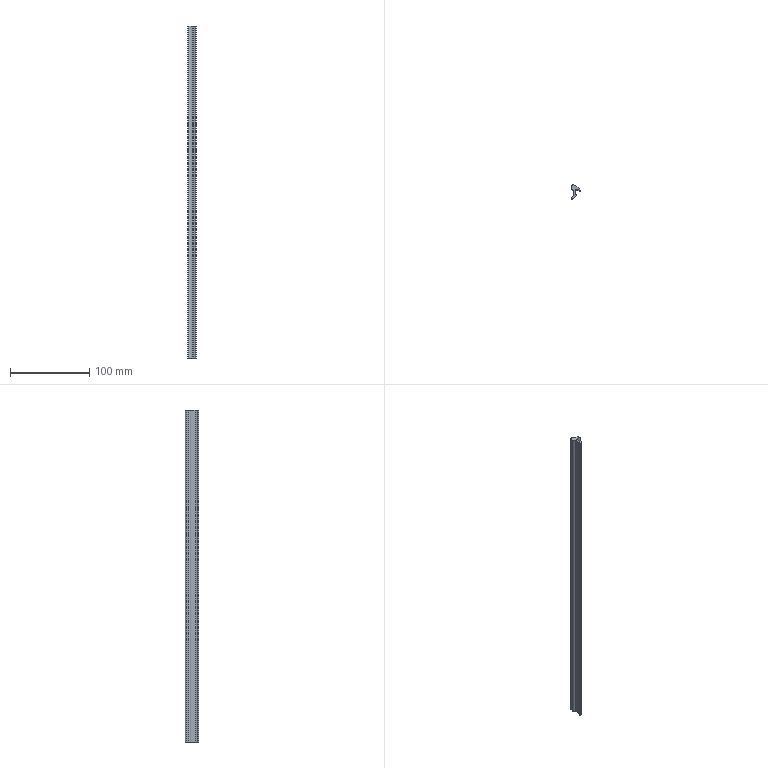Part | SolidWorks | features BaseBody 1, MoveFace 1 | 1 solid | 20 faces | box 10.8 x 17.5 x 419 mm | volume 33017 mm3 | cylinder 11 | plane 9 | commonest cylinder face diameters 1.6 x2 14 x2 0.4 x1 0.6 x1 0.8 x1 2.6 x1
STEP:
#1=CARTESIAN_POINT('',(-3.236,-11.055,319.));
#2=VERTEX_POINT('',#1);
#3=CARTESIAN_POINT('',(-4.3,-10.3,319.));
#4=VERTEX_POINT('',#3);
#5=CARTESIAN_POINT('',(-3.5,-10.3,319.));
#6=DIRECTION('',(0.,0.,-1.));
#7=DIRECTION('',(1.,0.,0.));
#8=AXIS2_PLACEMENT_3D('',#5,#6,#7);
#9=CIRCLE('',#8,0.8);
#10=EDGE_CURVE('',#2,#4,#9,.T.);
#11=ORIENTED_EDGE('',*,*,#10,.T.);
#12=CARTESIAN_POINT('',(-4.3,-10.3,-100.));
#13=VERTEX_POINT('',#12);
#14=CARTESIAN_POINT('',(-4.3,-10.3,-100.));
#15=DIRECTION('',(0.,0.,-1.));
#16=VECTOR('',#15,1000.);
#17=LINE('',#14,#16);
#18=EDGE_CURVE('',#4,#13,#17,.T.);
#19=ORIENTED_EDGE('',*,*,#18,.T.);
#20=CARTESIAN_POINT('',(-3.236,-11.055,-100.));
#21=VERTEX_POINT('',#20);
#22=CARTESIAN_POINT('',(-3.5,-10.3,-100.));
#23=DIRECTION('',(0.,0.,1.));
#24=DIRECTION('',(-1.,0.,0.));
#25=AXIS2_PLACEMENT_3D('',#22,#23,#24);
#26=CIRCLE('',#25,0.8);
#27=EDGE_CURVE('',#13,#21,#26,.T.);
#28=ORIENTED_EDGE('',*,*,#27,.T.);
#29=CARTESIAN_POINT('',(-3.236,-11.055,-100.));
#30=DIRECTION('',(0.,0.,-1.));
#31=VECTOR('',#30,1000.);
#32=LINE('',#29,#31);
#33=EDGE_CURVE('',#2,#21,#32,.T.);
#34=ORIENTED_EDGE('',*,*,#33,.F.);
#35=EDGE_LOOP('',(#11,#19,#28,#34));
#36=FACE_OUTER_BOUND('',#35,.T.);
#37=CARTESIAN_POINT('',(-3.5,-10.3,-100.));
#38=DIRECTION('',(0.,0.,-1.));
#39=DIRECTION('',(-1.,0.,0.));
#40=AXIS2_PLACEMENT_3D('',#37,#38,#39);
#41=CYLINDRICAL_SURFACE('',#40,0.8);
#42=ADVANCED_FACE('',(#36),#41,.T.);
#43=CARTESIAN_POINT('',(1.184,-6.397,-100.));
#44=VERTEX_POINT('',#43);
#45=CARTESIAN_POINT('',(-5.702,-4.29,-100.));
#46=DIRECTION('',(0.,0.,1.));
#47=DIRECTION('',(-1.,0.,0.));
#48=AXIS2_PLACEMENT_3D('',#45,#46,#47);
#49=CIRCLE('',#48,7.201);
#50=EDGE_CURVE('',#21,#44,#49,.T.);
#51=ORIENTED_EDGE('',*,*,#50,.T.);
#52=CARTESIAN_POINT('',(1.184,-6.397,319.));
#53=VERTEX_POINT('',#52);
#54=CARTESIAN_POINT('',(1.184,-6.397,-100.));
#55=DIRECTION('',(0.,0.,1.));
#56=VECTOR('',#55,1000.);
#57=LINE('',#54,#56);
#58=EDGE_CURVE('',#44,#53,#57,.T.);
#59=ORIENTED_EDGE('',*,*,#58,.T.);
#60=CARTESIAN_POINT('',(-5.702,-4.29,319.));
#61=DIRECTION('',(0.,0.,-1.));
#62=DIRECTION('',(1.,0.,0.));
#63=AXIS2_PLACEMENT_3D('',#60,#61,#62);
#64=CIRCLE('',#63,7.201);
#65=EDGE_CURVE('',#53,#2,#64,.T.);
#66=ORIENTED_EDGE('',*,*,#65,.T.);
#67=ORIENTED_EDGE('',*,*,#33,.T.);
#68=EDGE_LOOP('',(#51,#59,#66,#67));
#69=FACE_OUTER_BOUND('',#68,.T.);
#70=CARTESIAN_POINT('',(-5.702,-4.29,-100.));
#71=DIRECTION('',(0.,0.,-1.));
#72=DIRECTION('',(-1.,0.,0.));
#73=AXIS2_PLACEMENT_3D('',#70,#71,#72);
#74=CYLINDRICAL_SURFACE('',#73,7.201);
#75=ADVANCED_FACE('',(#69),#74,.T.);
#76=CARTESIAN_POINT('',(0.9,-6.,-100.));
#77=VERTEX_POINT('',#76);
#78=CARTESIAN_POINT('',(0.9,-6.3,-100.));
#79=DIRECTION('',(0.,0.,1.));
#80=DIRECTION('',(-1.,0.,0.));
#81=AXIS2_PLACEMENT_3D('',#78,#79,#80);
#82=CIRCLE('',#81,0.3);
#83=EDGE_CURVE('',#44,#77,#82,.T.);
#84=ORIENTED_EDGE('',*,*,#83,.T.);
#85=CARTESIAN_POINT('',(0.9,-6.,319.));
#86=VERTEX_POINT('',#85);
#87=CARTESIAN_POINT('',(0.9,-6.,-100.));
#88=DIRECTION('',(0.,0.,1.));
#89=VECTOR('',#88,1000.);
#90=LINE('',#87,#89);
#91=EDGE_CURVE('',#77,#86,#90,.T.);
#92=ORIENTED_EDGE('',*,*,#91,.T.);
#93=CARTESIAN_POINT('',(0.9,-6.3,319.));
#94=DIRECTION('',(0.,0.,-1.));
#95=DIRECTION('',(1.,0.,0.));
#96=AXIS2_PLACEMENT_3D('',#93,#94,#95);
#97=CIRCLE('',#96,0.3);
#98=EDGE_CURVE('',#86,#53,#97,.T.);
#99=ORIENTED_EDGE('',*,*,#98,.T.);
#100=ORIENTED_EDGE('',*,*,#58,.F.);
#101=EDGE_LOOP('',(#84,#92,#99,#100));
#102=FACE_OUTER_BOUND('',#101,.T.);
#103=CARTESIAN_POINT('',(0.9,-6.3,-100.));
#104=DIRECTION('',(0.,0.,-1.));
#105=DIRECTION('',(-1.,0.,0.));
#106=AXIS2_PLACEMENT_3D('',#103,#104,#105);
#107=CYLINDRICAL_SURFACE('',#106,0.3);
#108=ADVANCED_FACE('',(#102),#107,.T.);
#109=CARTESIAN_POINT('',(-2.5,-0.5,-100.));
#110=VERTEX_POINT('',#109);
#111=CARTESIAN_POINT('',(-2.5,-6.153,-100.));
#112=VERTEX_POINT('',#111);
#113=CARTESIAN_POINT('',(-2.5,-6.397,-100.));
#114=DIRECTION('',(0.,-1.,0.));
#115=VECTOR('',#114,1000.);
#116=LINE('',#113,#115);
#117=EDGE_CURVE('',#110,#112,#116,.T.);
#118=ORIENTED_EDGE('',*,*,#117,.F.);
#119=CARTESIAN_POINT('',(-4.2,1.695,-100.));
#120=VERTEX_POINT('',#119);
#121=CARTESIAN_POINT('',(-1.701,1.875,-100.));
#122=DIRECTION('',(0.,0.,1.));
#123=DIRECTION('',(-1.,0.,0.));
#124=AXIS2_PLACEMENT_3D('',#121,#122,#123);
#125=CIRCLE('',#124,2.506);
#126=EDGE_CURVE('',#120,#110,#125,.T.);
#127=ORIENTED_EDGE('',*,*,#126,.F.);
#128=CARTESIAN_POINT('',(-4.2,5.1,-100.));
#129=VERTEX_POINT('',#128);
#130=CARTESIAN_POINT('',(-4.2,-6.397,-100.));
#131=DIRECTION('',(0.,-1.,0.));
#132=VECTOR('',#131,1000.);
#133=LINE('',#130,#132);
#134=EDGE_CURVE('',#129,#120,#133,.T.);
#135=ORIENTED_EDGE('',*,*,#134,.F.);
#136=CARTESIAN_POINT('',(-2.892,6.4,-100.));
#137=VERTEX_POINT('',#136);
#138=CARTESIAN_POINT('',(-2.9,5.1,-100.));
#139=DIRECTION('',(0.,0.,1.));
#140=DIRECTION('',(-1.,0.,0.));
#141=AXIS2_PLACEMENT_3D('',#138,#139,#140);
#142=CIRCLE('',#141,1.3);
#143=EDGE_CURVE('',#137,#129,#142,.T.);
#144=ORIENTED_EDGE('',*,*,#143,.F.);
#145=CARTESIAN_POINT('',(0.5,5.5,-100.));
#146=VERTEX_POINT('',#145);
#147=CARTESIAN_POINT('',(-2.934,-0.5999,-100.));
#148=DIRECTION('',(0.,0.,1.));
#149=DIRECTION('',(-1.,0.,0.));
#150=AXIS2_PLACEMENT_3D('',#147,#148,#149);
#151=CIRCLE('',#150,7.);
#152=EDGE_CURVE('',#146,#137,#151,.T.);
#153=ORIENTED_EDGE('',*,*,#152,.F.);
#154=CARTESIAN_POINT('',(5.5,1.7,-100.));
#155=VERTEX_POINT('',#154);
#156=CARTESIAN_POINT('',(5.5,1.7,-100.));
#157=DIRECTION('',(-0.7962,0.6051,0.));
#158=VECTOR('',#157,1000.);
#159=LINE('',#156,#158);
#160=EDGE_CURVE('',#155,#146,#159,.T.);
#161=ORIENTED_EDGE('',*,*,#160,.F.);
#162=CARTESIAN_POINT('',(6.458,-0.2215,-100.));
#163=VERTEX_POINT('',#162);
#164=CARTESIAN_POINT('',(6.458,-0.2215,-100.));
#165=DIRECTION('',(-0.4462,0.8949,0.));
#166=VECTOR('',#165,1000.);
#167=LINE('',#164,#166);
#168=EDGE_CURVE('',#163,#155,#167,.T.);
#169=ORIENTED_EDGE('',*,*,#168,.F.);
#170=CARTESIAN_POINT('',(5.895,-0.7433,-100.));
#171=VERTEX_POINT('',#170);
#172=CARTESIAN_POINT('',(6.1,-0.4,-100.));
#173=DIRECTION('',(0.,0.,1.));
#174=DIRECTION('',(-1.,0.,0.));
#175=AXIS2_PLACEMENT_3D('',#172,#173,#174);
#176=CIRCLE('',#175,0.4);
#177=EDGE_CURVE('',#171,#163,#176,.T.);
#178=ORIENTED_EDGE('',*,*,#177,.F.);
#179=CARTESIAN_POINT('',(3.,0.,-100.));
#180=VERTEX_POINT('',#179);
#181=CARTESIAN_POINT('',(2.746,-6.995,-100.));
#182=DIRECTION('',(0.,0.,-1.));
#183=DIRECTION('',(-1.,0.,0.));
#184=AXIS2_PLACEMENT_3D('',#181,#182,#183);
#185=CIRCLE('',#184,7.);
#186=EDGE_CURVE('',#180,#171,#185,.T.);
#187=ORIENTED_EDGE('',*,*,#186,.F.);
#188=CARTESIAN_POINT('',(0.,0.,-100.));
#189=VERTEX_POINT('',#188);
#190=CARTESIAN_POINT('',(-6.814,0.,-100.));
#191=DIRECTION('',(1.,0.,0.));
#192=VECTOR('',#191,1000.);
#193=LINE('',#190,#192);
#194=EDGE_CURVE('',#189,#180,#193,.T.);
#195=ORIENTED_EDGE('',*,*,#194,.F.);
#196=CARTESIAN_POINT('',(0.,-5.8,-100.));
#197=VERTEX_POINT('',#196);
#198=CARTESIAN_POINT('',(0.,-6.397,-100.));
#199=DIRECTION('',(0.,1.,0.));
#200=VECTOR('',#199,1000.);
#201=LINE('',#198,#200);
#202=EDGE_CURVE('',#197,#189,#201,.T.);
#203=ORIENTED_EDGE('',*,*,#202,.F.);
#204=CARTESIAN_POINT('',(0.2,-6.,-100.));
#205=VERTEX_POINT('',#204);
#206=CARTESIAN_POINT('',(0.2,-5.8,-100.));
#207=DIRECTION('',(0.,0.,1.));
#208=DIRECTION('',(-1.,0.,0.));
#209=AXIS2_PLACEMENT_3D('',#206,#207,#208);
#210=CIRCLE('',#209,0.2);
#211=EDGE_CURVE('',#197,#205,#210,.T.);
#212=ORIENTED_EDGE('',*,*,#211,.T.);
#213=CARTESIAN_POINT('',(-6.814,-6.,-100.));
#214=DIRECTION('',(-1.,0.,0.));
#215=VECTOR('',#214,1000.);
#216=LINE('',#213,#215);
#217=EDGE_CURVE('',#77,#205,#216,.T.);
#218=ORIENTED_EDGE('',*,*,#217,.F.);
#219=ORIENTED_EDGE('',*,*,#83,.F.);
#220=ORIENTED_EDGE('',*,*,#50,.F.);
#221=ORIENTED_EDGE('',*,*,#27,.F.);
#222=CARTESIAN_POINT('',(-3.998,-9.674,-100.));
#223=VERTEX_POINT('',#222);
#224=CARTESIAN_POINT('',(-3.5,-10.3,-100.));
#225=DIRECTION('',(0.,0.,1.));
#226=DIRECTION('',(-1.,0.,0.));
#227=AXIS2_PLACEMENT_3D('',#224,#225,#226);
#228=CIRCLE('',#227,0.8);
#229=EDGE_CURVE('',#223,#13,#228,.T.);
#230=ORIENTED_EDGE('',*,*,#229,.F.);
#231=CARTESIAN_POINT('',(-6.814,-6.397,-100.));
#232=DIRECTION('',(0.,0.,-1.));
#233=DIRECTION('',(-1.,0.,0.));
#234=AXIS2_PLACEMENT_3D('',#231,#232,#233);
#235=CIRCLE('',#234,4.321);
#236=EDGE_CURVE('',#112,#223,#235,.T.);
#237=ORIENTED_EDGE('',*,*,#236,.F.);
#238=EDGE_LOOP('',(#118,#127,#135,#144,#153,#161,#169,#178,#187,#195,#203,#212,#218,#219,#220,#221,#230,#237));
#239=FACE_OUTER_BOUND('',#238,.T.);
#240=CARTESIAN_POINT('',(-6.814,-6.397,-100.));
#241=DIRECTION('',(0.,0.,1.));
#242=DIRECTION('',(1.,0.,0.));
#243=AXIS2_PLACEMENT_3D('',#240,#241,#242);
#244=PLANE('',#243);
#245=ADVANCED_FACE('',(#239),#244,.F.);
#246=ORIENTED_EDGE('',*,*,#18,.F.);
#247=CARTESIAN_POINT('',(-3.998,-9.674,319.));
#248=VERTEX_POINT('',#247);
#249=CARTESIAN_POINT('',(-3.5,-10.3,319.));
#250=DIRECTION('',(0.,0.,-1.));
#251=DIRECTION('',(1.,0.,0.));
#252=AXIS2_PLACEMENT_3D('',#249,#250,#251);
#253=CIRCLE('',#252,0.8);
#254=EDGE_CURVE('',#4,#248,#253,.T.);
#255=ORIENTED_EDGE('',*,*,#254,.T.);
#256=CARTESIAN_POINT('',(-3.998,-9.674,-100.));
#257=DIRECTION('',(0.,0.,-1.));
#258=VECTOR('',#257,1000.);
#259=LINE('',#256,#258);
#260=EDGE_CURVE('',#248,#223,#259,.T.);
#261=ORIENTED_EDGE('',*,*,#260,.T.);
#262=ORIENTED_EDGE('',*,*,#229,.T.);
#263=EDGE_LOOP('',(#246,#255,#261,#262));
#264=FACE_OUTER_BOUND('',#263,.T.);
#265=CARTESIAN_POINT('',(-3.5,-10.3,-100.));
#266=DIRECTION('',(0.,0.,-1.));
#267=DIRECTION('',(-1.,0.,0.));
#268=AXIS2_PLACEMENT_3D('',#265,#266,#267);
#269=CYLINDRICAL_SURFACE('',#268,0.8);
#270=ADVANCED_FACE('',(#264),#269,.T.);
#271=CARTESIAN_POINT('',(-4.2,1.695,319.));
#272=VERTEX_POINT('',#271);
#273=CARTESIAN_POINT('',(-2.5,-0.5,319.));
#274=VERTEX_POINT('',#273);
#275=CARTESIAN_POINT('',(-1.701,1.875,319.));
#276=DIRECTION('',(0.,0.,1.));
#277=DIRECTION('',(1.,0.,0.));
#278=AXIS2_PLACEMENT_3D('',#275,#276,#277);
#279=CIRCLE('',#278,2.506);
#280=EDGE_CURVE('',#272,#274,#279,.T.);
#281=ORIENTED_EDGE('',*,*,#280,.T.);
#282=CARTESIAN_POINT('',(-2.5,-6.153,319.));
#283=VERTEX_POINT('',#282);
#284=CARTESIAN_POINT('',(-2.5,-6.397,319.));
#285=DIRECTION('',(0.,-1.,0.));
#286=VECTOR('',#285,1000.);
#287=LINE('',#284,#286);
#288=EDGE_CURVE('',#274,#283,#287,.T.);
#289=ORIENTED_EDGE('',*,*,#288,.T.);
#290=CARTESIAN_POINT('',(-6.814,-6.397,319.));
#291=DIRECTION('',(0.,0.,-1.));
#292=DIRECTION('',(1.,0.,0.));
#293=AXIS2_PLACEMENT_3D('',#290,#291,#292);
#294=CIRCLE('',#293,4.321);
#295=EDGE_CURVE('',#283,#248,#294,.T.);
#296=ORIENTED_EDGE('',*,*,#295,.T.);
#297=ORIENTED_EDGE('',*,*,#254,.F.);
#298=ORIENTED_EDGE('',*,*,#10,.F.);
#299=ORIENTED_EDGE('',*,*,#65,.F.);
#300=ORIENTED_EDGE('',*,*,#98,.F.);
#301=CARTESIAN_POINT('',(0.2,-6.,319.));
#302=VERTEX_POINT('',#301);
#303=CARTESIAN_POINT('',(-6.814,-6.,319.));
#304=DIRECTION('',(-1.,0.,0.));
#305=VECTOR('',#304,1000.);
#306=LINE('',#303,#305);
#307=EDGE_CURVE('',#86,#302,#306,.T.);
#308=ORIENTED_EDGE('',*,*,#307,.T.);
#309=CARTESIAN_POINT('',(0.,-5.8,319.));
#310=VERTEX_POINT('',#309);
#311=CARTESIAN_POINT('',(0.2,-5.8,319.));
#312=DIRECTION('',(0.,0.,-1.));
#313=DIRECTION('',(1.,0.,0.));
#314=AXIS2_PLACEMENT_3D('',#311,#312,#313);
#315=CIRCLE('',#314,0.2);
#316=EDGE_CURVE('',#302,#310,#315,.T.);
#317=ORIENTED_EDGE('',*,*,#316,.T.);
#318=CARTESIAN_POINT('',(0.,0.,319.));
#319=VERTEX_POINT('',#318);
#320=CARTESIAN_POINT('',(0.,-6.397,319.));
#321=DIRECTION('',(0.,1.,0.));
#322=VECTOR('',#321,1000.);
#323=LINE('',#320,#322);
#324=EDGE_CURVE('',#310,#319,#323,.T.);
#325=ORIENTED_EDGE('',*,*,#324,.T.);
#326=CARTESIAN_POINT('',(3.,0.,319.));
#327=VERTEX_POINT('',#326);
#328=CARTESIAN_POINT('',(-6.814,0.,319.));
#329=DIRECTION('',(1.,0.,0.));
#330=VECTOR('',#329,1000.);
#331=LINE('',#328,#330);
#332=EDGE_CURVE('',#319,#327,#331,.T.);
#333=ORIENTED_EDGE('',*,*,#332,.T.);
#334=CARTESIAN_POINT('',(5.895,-0.7433,319.));
#335=VERTEX_POINT('',#334);
#336=CARTESIAN_POINT('',(2.746,-6.995,319.));
#337=DIRECTION('',(0.,0.,-1.));
#338=DIRECTION('',(1.,0.,0.));
#339=AXIS2_PLACEMENT_3D('',#336,#337,#338);
#340=CIRCLE('',#339,7.);
#341=EDGE_CURVE('',#327,#335,#340,.T.);
#342=ORIENTED_EDGE('',*,*,#341,.T.);
#343=CARTESIAN_POINT('',(6.458,-0.2215,319.));
#344=VERTEX_POINT('',#343);
#345=CARTESIAN_POINT('',(6.1,-0.4,319.));
#346=DIRECTION('',(0.,0.,-1.));
#347=DIRECTION('',(1.,0.,0.));
#348=AXIS2_PLACEMENT_3D('',#345,#346,#347);
#349=CIRCLE('',#348,0.4);
#350=EDGE_CURVE('',#344,#335,#349,.T.);
#351=ORIENTED_EDGE('',*,*,#350,.F.);
#352=CARTESIAN_POINT('',(5.5,1.7,319.));
#353=VERTEX_POINT('',#352);
#354=CARTESIAN_POINT('',(6.282,0.1323,319.));
#355=DIRECTION('',(-0.4462,0.8949,0.));
#356=VECTOR('',#355,1000.);
#357=LINE('',#354,#356);
#358=EDGE_CURVE('',#344,#353,#357,.T.);
#359=ORIENTED_EDGE('',*,*,#358,.T.);
#360=CARTESIAN_POINT('',(0.5,5.5,319.));
#361=VERTEX_POINT('',#360);
#362=CARTESIAN_POINT('',(1.595,4.668,319.));
#363=DIRECTION('',(-0.7962,0.6051,0.));
#364=VECTOR('',#363,1000.);
#365=LINE('',#362,#364);
#366=EDGE_CURVE('',#353,#361,#365,.T.);
#367=ORIENTED_EDGE('',*,*,#366,.T.);
#368=CARTESIAN_POINT('',(-2.892,6.4,319.));
#369=VERTEX_POINT('',#368);
#370=CARTESIAN_POINT('',(-2.934,-0.5999,319.));
#371=DIRECTION('',(0.,0.,1.));
#372=DIRECTION('',(1.,0.,0.));
#373=AXIS2_PLACEMENT_3D('',#370,#371,#372);
#374=CIRCLE('',#373,7.);
#375=EDGE_CURVE('',#361,#369,#374,.T.);
#376=ORIENTED_EDGE('',*,*,#375,.T.);
#377=CARTESIAN_POINT('',(-4.2,5.1,319.));
#378=VERTEX_POINT('',#377);
#379=CARTESIAN_POINT('',(-2.9,5.1,319.));
#380=DIRECTION('',(0.,0.,1.));
#381=DIRECTION('',(1.,0.,0.));
#382=AXIS2_PLACEMENT_3D('',#379,#380,#381);
#383=CIRCLE('',#382,1.3);
#384=EDGE_CURVE('',#369,#378,#383,.T.);
#385=ORIENTED_EDGE('',*,*,#384,.T.);
#386=CARTESIAN_POINT('',(-4.2,-6.397,319.));
#387=DIRECTION('',(0.,-1.,0.));
#388=VECTOR('',#387,1000.);
#389=LINE('',#386,#388);
#390=EDGE_CURVE('',#378,#272,#389,.T.);
#391=ORIENTED_EDGE('',*,*,#390,.T.);
#392=EDGE_LOOP('',(#281,#289,#296,#297,#298,#299,#300,#308,#317,#325,#333,#342,#351,#359,#367,#376,#385,#391));
#393=FACE_OUTER_BOUND('',#392,.T.);
#394=CARTESIAN_POINT('',(-6.814,-6.397,319.));
#395=DIRECTION('',(0.,0.,1.));
#396=DIRECTION('',(1.,0.,0.));
#397=AXIS2_PLACEMENT_3D('',#394,#395,#396);
#398=PLANE('',#397);
#399=ADVANCED_FACE('',(#393),#398,.T.);
#400=ORIENTED_EDGE('',*,*,#217,.T.);
#401=CARTESIAN_POINT('',(0.2,-6.,-100.));
#402=DIRECTION('',(0.,0.,1.));
#403=VECTOR('',#402,1000.);
#404=LINE('',#401,#403);
#405=EDGE_CURVE('',#205,#302,#404,.T.);
#406=ORIENTED_EDGE('',*,*,#405,.T.);
#407=ORIENTED_EDGE('',*,*,#307,.F.);
#408=ORIENTED_EDGE('',*,*,#91,.F.);
#409=EDGE_LOOP('',(#400,#406,#407,#408));
#410=FACE_OUTER_BOUND('',#409,.T.);
#411=CARTESIAN_POINT('',(0.9,-6.,-100.));
#412=DIRECTION('',(0.,1.,0.));
#413=DIRECTION('',(0.,0.,1.));
#414=AXIS2_PLACEMENT_3D('',#411,#412,#413);
#415=PLANE('',#414);
#416=ADVANCED_FACE('',(#410),#415,.T.);
#417=CARTESIAN_POINT('',(-2.5,-6.153,-100.));
#418=DIRECTION('',(0.,0.,1.));
#419=VECTOR('',#418,1000.);
#420=LINE('',#417,#419);
#421=EDGE_CURVE('',#112,#283,#420,.T.);
#422=ORIENTED_EDGE('',*,*,#421,.F.);
#423=ORIENTED_EDGE('',*,*,#236,.T.);
#424=ORIENTED_EDGE('',*,*,#260,.F.);
#425=ORIENTED_EDGE('',*,*,#295,.F.);
#426=EDGE_LOOP('',(#422,#423,#424,#425));
#427=FACE_OUTER_BOUND('',#426,.T.);
#428=CARTESIAN_POINT('',(-6.814,-6.397,-100.));
#429=DIRECTION('',(0.,0.,-1.));
#430=DIRECTION('',(-1.,0.,0.));
#431=AXIS2_PLACEMENT_3D('',#428,#429,#430);
#432=CYLINDRICAL_SURFACE('',#431,4.321);
#433=ADVANCED_FACE('',(#427),#432,.F.);
#434=ORIENTED_EDGE('',*,*,#117,.T.);
#435=ORIENTED_EDGE('',*,*,#421,.T.);
#436=ORIENTED_EDGE('',*,*,#288,.F.);
#437=CARTESIAN_POINT('',(-2.5,-0.5,-100.));
#438=DIRECTION('',(0.,0.,-1.));
#439=VECTOR('',#438,1000.);
#440=LINE('',#437,#439);
#441=EDGE_CURVE('',#274,#110,#440,.T.);
#442=ORIENTED_EDGE('',*,*,#441,.T.);
#443=EDGE_LOOP('',(#434,#435,#436,#442));
#444=FACE_OUTER_BOUND('',#443,.T.);
#445=CARTESIAN_POINT('',(-2.5,-0.5,-100.));
#446=DIRECTION('',(-1.,0.,0.));
#447=DIRECTION('',(0.,0.,1.));
#448=AXIS2_PLACEMENT_3D('',#445,#446,#447);
#449=PLANE('',#448);
#450=ADVANCED_FACE('',(#444),#449,.T.);
#451=ORIENTED_EDGE('',*,*,#126,.T.);
#452=ORIENTED_EDGE('',*,*,#441,.F.);
#453=ORIENTED_EDGE('',*,*,#280,.F.);
#454=CARTESIAN_POINT('',(-4.2,1.695,-100.));
#455=DIRECTION('',(0.,0.,-1.));
#456=VECTOR('',#455,1000.);
#457=LINE('',#454,#456);
#458=EDGE_CURVE('',#272,#120,#457,.T.);
#459=ORIENTED_EDGE('',*,*,#458,.T.);
#460=EDGE_LOOP('',(#451,#452,#453,#459));
#461=FACE_OUTER_BOUND('',#460,.T.);
#462=CARTESIAN_POINT('',(-1.701,1.875,-100.));
#463=DIRECTION('',(0.,0.,-1.));
#464=DIRECTION('',(-1.,0.,0.));
#465=AXIS2_PLACEMENT_3D('',#462,#463,#464);
#466=CYLINDRICAL_SURFACE('',#465,2.506);
#467=ADVANCED_FACE('',(#461),#466,.T.);
#468=ORIENTED_EDGE('',*,*,#134,.T.);
#469=ORIENTED_EDGE('',*,*,#458,.F.);
#470=ORIENTED_EDGE('',*,*,#390,.F.);
#471=CARTESIAN_POINT('',(-4.2,5.1,-100.));
#472=DIRECTION('',(0.,0.,-1.));
#473=VECTOR('',#472,1000.);
#474=LINE('',#471,#473);
#475=EDGE_CURVE('',#378,#129,#474,.T.);
#476=ORIENTED_EDGE('',*,*,#475,.T.);
#477=EDGE_LOOP('',(#468,#469,#470,#476));
#478=FACE_OUTER_BOUND('',#477,.T.);
#479=CARTESIAN_POINT('',(-4.2,5.1,-100.));
#480=DIRECTION('',(-1.,0.,0.));
#481=DIRECTION('',(0.,0.,1.));
#482=AXIS2_PLACEMENT_3D('',#479,#480,#481);
#483=PLANE('',#482);
#484=ADVANCED_FACE('',(#478),#483,.T.);
#485=ORIENTED_EDGE('',*,*,#143,.T.);
#486=ORIENTED_EDGE('',*,*,#475,.F.);
#487=ORIENTED_EDGE('',*,*,#384,.F.);
#488=CARTESIAN_POINT('',(-2.892,6.4,-100.));
#489=DIRECTION('',(0.,0.,-1.));
#490=VECTOR('',#489,1000.);
#491=LINE('',#488,#490);
#492=EDGE_CURVE('',#369,#137,#491,.T.);
#493=ORIENTED_EDGE('',*,*,#492,.T.);
#494=EDGE_LOOP('',(#485,#486,#487,#493));
#495=FACE_OUTER_BOUND('',#494,.T.);
#496=CARTESIAN_POINT('',(-2.9,5.1,-100.));
#497=DIRECTION('',(0.,0.,-1.));
#498=DIRECTION('',(-1.,0.,0.));
#499=AXIS2_PLACEMENT_3D('',#496,#497,#498);
#500=CYLINDRICAL_SURFACE('',#499,1.3);
#501=ADVANCED_FACE('',(#495),#500,.T.);
#502=ORIENTED_EDGE('',*,*,#152,.T.);
#503=ORIENTED_EDGE('',*,*,#492,.F.);
#504=ORIENTED_EDGE('',*,*,#375,.F.);
#505=CARTESIAN_POINT('',(0.5,5.5,-100.));
#506=DIRECTION('',(0.,0.,-1.));
#507=VECTOR('',#506,1000.);
#508=LINE('',#505,#507);
#509=EDGE_CURVE('',#361,#146,#508,.T.);
#510=ORIENTED_EDGE('',*,*,#509,.T.);
#511=EDGE_LOOP('',(#502,#503,#504,#510));
#512=FACE_OUTER_BOUND('',#511,.T.);
#513=CARTESIAN_POINT('',(-2.934,-0.5999,-100.));
#514=DIRECTION('',(0.,0.,-1.));
#515=DIRECTION('',(-1.,0.,0.));
#516=AXIS2_PLACEMENT_3D('',#513,#514,#515);
#517=CYLINDRICAL_SURFACE('',#516,7.);
#518=ADVANCED_FACE('',(#512),#517,.T.);
#519=ORIENTED_EDGE('',*,*,#160,.T.);
#520=ORIENTED_EDGE('',*,*,#509,.F.);
#521=ORIENTED_EDGE('',*,*,#366,.F.);
#522=CARTESIAN_POINT('',(5.5,1.7,-100.));
#523=DIRECTION('',(0.,0.,-1.));
#524=VECTOR('',#523,1000.);
#525=LINE('',#522,#524);
#526=EDGE_CURVE('',#353,#155,#525,.T.);
#527=ORIENTED_EDGE('',*,*,#526,.T.);
#528=EDGE_LOOP('',(#519,#520,#521,#527));
#529=FACE_OUTER_BOUND('',#528,.T.);
#530=CARTESIAN_POINT('',(5.5,1.7,-100.));
#531=DIRECTION('',(0.6051,0.7962,0.));
#532=DIRECTION('',(-0.7962,0.6051,0.));
#533=AXIS2_PLACEMENT_3D('',#530,#531,#532);
#534=PLANE('',#533);
#535=ADVANCED_FACE('',(#529),#534,.T.);
#536=ORIENTED_EDGE('',*,*,#168,.T.);
#537=ORIENTED_EDGE('',*,*,#526,.F.);
#538=ORIENTED_EDGE('',*,*,#358,.F.);
#539=CARTESIAN_POINT('',(6.458,-0.2215,-100.));
#540=DIRECTION('',(0.,0.,-1.));
#541=VECTOR('',#540,1000.);
#542=LINE('',#539,#541);
#543=EDGE_CURVE('',#344,#163,#542,.T.);
#544=ORIENTED_EDGE('',*,*,#543,.T.);
#545=EDGE_LOOP('',(#536,#537,#538,#544));
#546=FACE_OUTER_BOUND('',#545,.T.);
#547=CARTESIAN_POINT('',(6.458,-0.2215,-100.));
#548=DIRECTION('',(0.8949,0.4462,0.));
#549=DIRECTION('',(-0.4462,0.8949,0.));
#550=AXIS2_PLACEMENT_3D('',#547,#548,#549);
#551=PLANE('',#550);
#552=ADVANCED_FACE('',(#546),#551,.T.);
#553=CARTESIAN_POINT('',(3.,0.,-100.));
#554=DIRECTION('',(0.,0.,1.));
#555=VECTOR('',#554,1000.);
#556=LINE('',#553,#555);
#557=EDGE_CURVE('',#180,#327,#556,.T.);
#558=ORIENTED_EDGE('',*,*,#557,.F.);
#559=ORIENTED_EDGE('',*,*,#186,.T.);
#560=CARTESIAN_POINT('',(5.895,-0.7433,-100.));
#561=DIRECTION('',(0.,0.,-1.));
#562=VECTOR('',#561,1000.);
#563=LINE('',#560,#562);
#564=EDGE_CURVE('',#335,#171,#563,.T.);
#565=ORIENTED_EDGE('',*,*,#564,.F.);
#566=ORIENTED_EDGE('',*,*,#341,.F.);
#567=EDGE_LOOP('',(#558,#559,#565,#566));
#568=FACE_OUTER_BOUND('',#567,.T.);
#569=CARTESIAN_POINT('',(2.746,-6.995,-100.));
#570=DIRECTION('',(0.,0.,-1.));
#571=DIRECTION('',(-1.,0.,0.));
#572=AXIS2_PLACEMENT_3D('',#569,#570,#571);
#573=CYLINDRICAL_SURFACE('',#572,7.);
#574=ADVANCED_FACE('',(#568),#573,.F.);
#575=ORIENTED_EDGE('',*,*,#194,.T.);
#576=ORIENTED_EDGE('',*,*,#557,.T.);
#577=ORIENTED_EDGE('',*,*,#332,.F.);
#578=CARTESIAN_POINT('',(0.,0.,-100.));
#579=DIRECTION('',(0.,0.,-1.));
#580=VECTOR('',#579,1000.);
#581=LINE('',#578,#580);
#582=EDGE_CURVE('',#319,#189,#581,.T.);
#583=ORIENTED_EDGE('',*,*,#582,.T.);
#584=EDGE_LOOP('',(#575,#576,#577,#583));
#585=FACE_OUTER_BOUND('',#584,.T.);
#586=CARTESIAN_POINT('',(0.,0.,-100.));
#587=DIRECTION('',(0.,-1.,0.));
#588=DIRECTION('',(0.,0.,-1.));
#589=AXIS2_PLACEMENT_3D('',#586,#587,#588);
#590=PLANE('',#589);
#591=ADVANCED_FACE('',(#585),#590,.T.);
#592=ORIENTED_EDGE('',*,*,#202,.T.);
#593=ORIENTED_EDGE('',*,*,#582,.F.);
#594=ORIENTED_EDGE('',*,*,#324,.F.);
#595=CARTESIAN_POINT('',(0.,-5.8,-100.));
#596=DIRECTION('',(0.,0.,-1.));
#597=VECTOR('',#596,1000.);
#598=LINE('',#595,#597);
#599=EDGE_CURVE('',#310,#197,#598,.T.);
#600=ORIENTED_EDGE('',*,*,#599,.T.);
#601=EDGE_LOOP('',(#592,#593,#594,#600));
#602=FACE_OUTER_BOUND('',#601,.T.);
#603=CARTESIAN_POINT('',(0.,-5.8,-100.));
#604=DIRECTION('',(1.,0.,0.));
#605=DIRECTION('',(0.,0.,-1.));
#606=AXIS2_PLACEMENT_3D('',#603,#604,#605);
#607=PLANE('',#606);
#608=ADVANCED_FACE('',(#602),#607,.T.);
#609=ORIENTED_EDGE('',*,*,#405,.F.);
#610=ORIENTED_EDGE('',*,*,#211,.F.);
#611=ORIENTED_EDGE('',*,*,#599,.F.);
#612=ORIENTED_EDGE('',*,*,#316,.F.);
#613=EDGE_LOOP('',(#609,#610,#611,#612));
#614=FACE_OUTER_BOUND('',#613,.T.);
#615=CARTESIAN_POINT('',(0.2,-5.8,-100.));
#616=DIRECTION('',(0.,0.,-1.));
#617=DIRECTION('',(-1.,0.,0.));
#618=AXIS2_PLACEMENT_3D('',#615,#616,#617);
#619=CYLINDRICAL_SURFACE('',#618,0.2);
#620=ADVANCED_FACE('',(#614),#619,.F.);
#621=ORIENTED_EDGE('',*,*,#177,.T.);
#622=ORIENTED_EDGE('',*,*,#543,.F.);
#623=ORIENTED_EDGE('',*,*,#350,.T.);
#624=ORIENTED_EDGE('',*,*,#564,.T.);
#625=EDGE_LOOP('',(#621,#622,#623,#624));
#626=FACE_OUTER_BOUND('',#625,.T.);
#627=CARTESIAN_POINT('',(6.1,-0.4,-100.));
#628=DIRECTION('',(0.,0.,-1.));
#629=DIRECTION('',(-1.,0.,0.));
#630=AXIS2_PLACEMENT_3D('',#627,#628,#629);
#631=CYLINDRICAL_SURFACE('',#630,0.4);
#632=ADVANCED_FACE('',(#626),#631,.T.);
#633=CLOSED_SHELL('',(#42,#75,#108,#245,#270,#399,#416,#433,#450,#467,#484,#501,#518,#535,#552,#574,#591,#608,#620,#632));
#634=MANIFOLD_SOLID_BREP('',#633);
#635=CARTESIAN_POINT('',(0.,0.,0.));
#636=DIRECTION('',(0.,0.,1.));
#637=DIRECTION('',(1.,0.,0.));
#638=AXIS2_PLACEMENT_3D('',#635,#636,#637);
#639=(LENGTH_UNIT()NAMED_UNIT(*)SI_UNIT(.MILLI.,.METRE.));
#640=UNCERTAINTY_MEASURE_WITH_UNIT(LENGTH_MEASURE(0.00001),#639,'','');
#641=(NAMED_UNIT(*)PLANE_ANGLE_UNIT()SI_UNIT($,.RADIAN.));
#642=(NAMED_UNIT(*)SI_UNIT($,.STERADIAN.)SOLID_ANGLE_UNIT());
#643=(GEOMETRIC_REPRESENTATION_CONTEXT(3)GLOBAL_UNCERTAINTY_ASSIGNED_CONTEXT((#640))GLOBAL_UNIT_ASSIGNED_CONTEXT((#639,#641,#642))REPRESENTATION_CONTEXT('',''));
#644=ADVANCED_BREP_SHAPE_REPRESENTATION('',(#634,#638),#643);